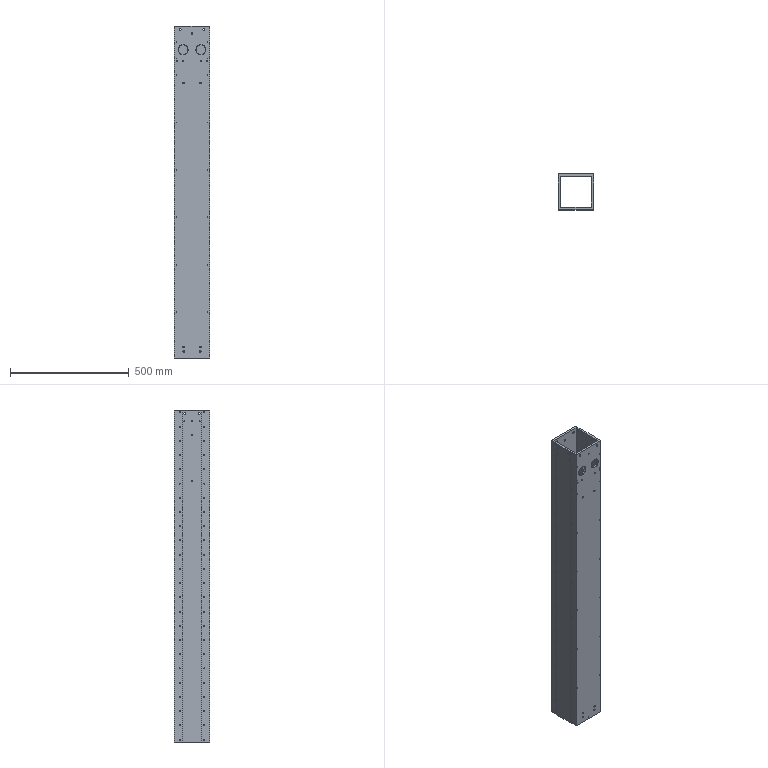Part | SolidWorks | features HoleWzd 12, ICE 2, Chamfer 1, Cut 1, Extrusion 1, Fillet 1 | 1 solid | 392 faces | box 150 x 150 x 1400 mm | volume 7296218 mm3 | cylinder 312 | cone 56 | plane 24 | commonest cylinder face diameters 4.2 x212 3.3 x44 6.8 x16 8.5 x16 5 x12 6 x4